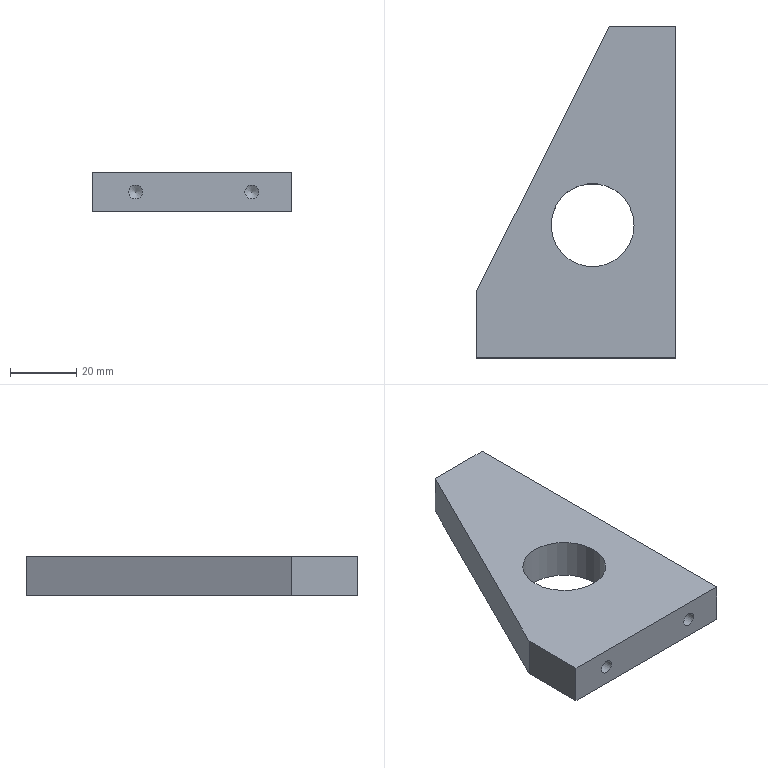Part | NX | 1 solid | 16 faces | box 60 x 100 x 12 mm | volume 45901 mm3 | plane 7 | cylinder 5 | cone 4 | commonest cylinder face diameters 4.2 x2 5 x2 25 x1
STEP:
#1=CARTESIAN_POINT('',(-30.,-30.,6.));
#2=VERTEX_POINT('',#1);
#3=CARTESIAN_POINT('',(-30.,-50.,6.));
#4=VERTEX_POINT('',#3);
#5=CARTESIAN_POINT('',(-30.,50.,6.));
#6=DIRECTION('',(0.,-1.,0.));
#7=VECTOR('',#6,1000.);
#8=LINE('',#5,#7);
#9=EDGE_CURVE('',#2,#4,#8,.T.);
#10=ORIENTED_EDGE('',*,*,#9,.F.);
#11=CARTESIAN_POINT('',(-30.,-30.,-6.));
#12=VERTEX_POINT('',#11);
#13=CARTESIAN_POINT('',(-30.,-30.,6.));
#14=DIRECTION('',(0.,0.,-1.));
#15=VECTOR('',#14,1000.);
#16=LINE('',#13,#15);
#17=EDGE_CURVE('',#2,#12,#16,.T.);
#18=ORIENTED_EDGE('',*,*,#17,.T.);
#19=CARTESIAN_POINT('',(-30.,-50.,-6.));
#20=VERTEX_POINT('',#19);
#21=CARTESIAN_POINT('',(-30.,50.,-6.));
#22=DIRECTION('',(0.,-1.,0.));
#23=VECTOR('',#22,1000.);
#24=LINE('',#21,#23);
#25=EDGE_CURVE('',#12,#20,#24,.T.);
#26=ORIENTED_EDGE('',*,*,#25,.T.);
#27=CARTESIAN_POINT('',(-30.,-50.,6.));
#28=DIRECTION('',(0.,0.,-1.));
#29=VECTOR('',#28,1000.);
#30=LINE('',#27,#29);
#31=EDGE_CURVE('',#4,#20,#30,.T.);
#32=ORIENTED_EDGE('',*,*,#31,.F.);
#33=EDGE_LOOP('',(#10,#18,#26,#32));
#34=FACE_BOUND('',#33,.T.);
#35=CARTESIAN_POINT('',(-30.,50.,6.));
#36=DIRECTION('',(1.,0.,0.));
#37=DIRECTION('',(0.,1.,0.));
#38=AXIS2_PLACEMENT_3D('',#35,#36,#37);
#39=PLANE('',#38);
#40=ADVANCED_FACE('',(#34),#39,.F.);
#41=CARTESIAN_POINT('',(18.,-50.,-2.1));
#42=VERTEX_POINT('',#41);
#43=CARTESIAN_POINT('',(18.,-50.,0.));
#44=DIRECTION('',(0.,-1.,0.));
#45=DIRECTION('',(0.,0.,-1.));
#46=AXIS2_PLACEMENT_3D('',#43,#44,#45);
#47=CIRCLE('',#46,2.1);
#48=EDGE_CURVE('',#42,#42,#47,.T.);
#49=ORIENTED_EDGE('',*,*,#48,.F.);
#50=EDGE_LOOP('',(#49));
#51=FACE_BOUND('',#50,.T.);
#52=CARTESIAN_POINT('',(-17.,-50.,-2.1));
#53=VERTEX_POINT('',#52);
#54=CARTESIAN_POINT('',(-17.,-50.,0.));
#55=DIRECTION('',(0.,-1.,0.));
#56=DIRECTION('',(0.,0.,-1.));
#57=AXIS2_PLACEMENT_3D('',#54,#55,#56);
#58=CIRCLE('',#57,2.1);
#59=EDGE_CURVE('',#53,#53,#58,.T.);
#60=ORIENTED_EDGE('',*,*,#59,.F.);
#61=EDGE_LOOP('',(#60));
#62=FACE_BOUND('',#61,.T.);
#63=CARTESIAN_POINT('',(30.,-50.,-6.));
#64=VERTEX_POINT('',#63);
#65=CARTESIAN_POINT('',(30.,-50.,-6.));
#66=DIRECTION('',(1.,0.,0.));
#67=VECTOR('',#66,1000.);
#68=LINE('',#65,#67);
#69=EDGE_CURVE('',#20,#64,#68,.T.);
#70=ORIENTED_EDGE('',*,*,#69,.T.);
#71=CARTESIAN_POINT('',(30.,-50.,6.));
#72=VERTEX_POINT('',#71);
#73=CARTESIAN_POINT('',(30.,-50.,6.));
#74=DIRECTION('',(0.,0.,-1.));
#75=VECTOR('',#74,1000.);
#76=LINE('',#73,#75);
#77=EDGE_CURVE('',#72,#64,#76,.T.);
#78=ORIENTED_EDGE('',*,*,#77,.F.);
#79=CARTESIAN_POINT('',(30.,-50.,6.));
#80=DIRECTION('',(1.,0.,0.));
#81=VECTOR('',#80,1000.);
#82=LINE('',#79,#81);
#83=EDGE_CURVE('',#4,#72,#82,.T.);
#84=ORIENTED_EDGE('',*,*,#83,.F.);
#85=ORIENTED_EDGE('',*,*,#31,.T.);
#86=EDGE_LOOP('',(#70,#78,#84,#85));
#87=FACE_BOUND('',#86,.T.);
#88=CARTESIAN_POINT('',(30.,-50.,6.));
#89=DIRECTION('',(0.,1.,0.));
#90=DIRECTION('',(-1.,0.,0.));
#91=AXIS2_PLACEMENT_3D('',#88,#89,#90);
#92=PLANE('',#91);
#93=ADVANCED_FACE('',(#51,#62,#87),#92,.F.);
#94=CARTESIAN_POINT('',(30.,35.,-2.5));
#95=VERTEX_POINT('',#94);
#96=CARTESIAN_POINT('',(30.,35.,0.));
#97=DIRECTION('',(1.,0.,0.));
#98=DIRECTION('',(0.,0.,-1.));
#99=AXIS2_PLACEMENT_3D('',#96,#97,#98);
#100=CIRCLE('',#99,2.5);
#101=EDGE_CURVE('',#95,#95,#100,.T.);
#102=ORIENTED_EDGE('',*,*,#101,.F.);
#103=EDGE_LOOP('',(#102));
#104=FACE_BOUND('',#103,.T.);
#105=CARTESIAN_POINT('',(30.,-30.,-2.5));
#106=VERTEX_POINT('',#105);
#107=CARTESIAN_POINT('',(30.,-30.,0.));
#108=DIRECTION('',(1.,0.,0.));
#109=DIRECTION('',(0.,0.,-1.));
#110=AXIS2_PLACEMENT_3D('',#107,#108,#109);
#111=CIRCLE('',#110,2.5);
#112=EDGE_CURVE('',#106,#106,#111,.T.);
#113=ORIENTED_EDGE('',*,*,#112,.F.);
#114=EDGE_LOOP('',(#113));
#115=FACE_BOUND('',#114,.T.);
#116=CARTESIAN_POINT('',(30.,50.,-6.));
#117=VERTEX_POINT('',#116);
#118=CARTESIAN_POINT('',(30.,50.,-6.));
#119=DIRECTION('',(0.,1.,0.));
#120=VECTOR('',#119,1000.);
#121=LINE('',#118,#120);
#122=EDGE_CURVE('',#64,#117,#121,.T.);
#123=ORIENTED_EDGE('',*,*,#122,.T.);
#124=CARTESIAN_POINT('',(30.,50.,6.));
#125=VERTEX_POINT('',#124);
#126=CARTESIAN_POINT('',(30.,50.,6.));
#127=DIRECTION('',(0.,0.,-1.));
#128=VECTOR('',#127,1000.);
#129=LINE('',#126,#128);
#130=EDGE_CURVE('',#125,#117,#129,.T.);
#131=ORIENTED_EDGE('',*,*,#130,.F.);
#132=CARTESIAN_POINT('',(30.,50.,6.));
#133=DIRECTION('',(0.,1.,0.));
#134=VECTOR('',#133,1000.);
#135=LINE('',#132,#134);
#136=EDGE_CURVE('',#72,#125,#135,.T.);
#137=ORIENTED_EDGE('',*,*,#136,.F.);
#138=ORIENTED_EDGE('',*,*,#77,.T.);
#139=EDGE_LOOP('',(#123,#131,#137,#138));
#140=FACE_BOUND('',#139,.T.);
#141=CARTESIAN_POINT('',(30.,50.,6.));
#142=DIRECTION('',(-1.,0.,0.));
#143=DIRECTION('',(0.,-1.,0.));
#144=AXIS2_PLACEMENT_3D('',#141,#142,#143);
#145=PLANE('',#144);
#146=ADVANCED_FACE('',(#104,#115,#140),#145,.F.);
#147=CARTESIAN_POINT('',(10.,50.,-6.));
#148=VERTEX_POINT('',#147);
#149=CARTESIAN_POINT('',(30.,50.,-6.));
#150=DIRECTION('',(-1.,0.,0.));
#151=VECTOR('',#150,1000.);
#152=LINE('',#149,#151);
#153=EDGE_CURVE('',#117,#148,#152,.T.);
#154=ORIENTED_EDGE('',*,*,#153,.T.);
#155=CARTESIAN_POINT('',(10.,50.,6.));
#156=VERTEX_POINT('',#155);
#157=CARTESIAN_POINT('',(10.,50.,6.));
#158=DIRECTION('',(0.,0.,1.));
#159=VECTOR('',#158,1000.);
#160=LINE('',#157,#159);
#161=EDGE_CURVE('',#148,#156,#160,.T.);
#162=ORIENTED_EDGE('',*,*,#161,.T.);
#163=CARTESIAN_POINT('',(30.,50.,6.));
#164=DIRECTION('',(-1.,0.,0.));
#165=VECTOR('',#164,1000.);
#166=LINE('',#163,#165);
#167=EDGE_CURVE('',#125,#156,#166,.T.);
#168=ORIENTED_EDGE('',*,*,#167,.F.);
#169=ORIENTED_EDGE('',*,*,#130,.T.);
#170=EDGE_LOOP('',(#154,#162,#168,#169));
#171=FACE_BOUND('',#170,.T.);
#172=CARTESIAN_POINT('',(30.,50.,6.));
#173=DIRECTION('',(0.,-1.,0.));
#174=DIRECTION('',(1.,0.,0.));
#175=AXIS2_PLACEMENT_3D('',#172,#173,#174);
#176=PLANE('',#175);
#177=ADVANCED_FACE('',(#171),#176,.F.);
#178=CARTESIAN_POINT('',(17.5,-10.,6.));
#179=VERTEX_POINT('',#178);
#180=CARTESIAN_POINT('',(5.,-10.,6.));
#181=DIRECTION('',(0.,0.,1.));
#182=DIRECTION('',(1.,0.,0.));
#183=AXIS2_PLACEMENT_3D('',#180,#181,#182);
#184=CIRCLE('',#183,12.5);
#185=EDGE_CURVE('',#179,#179,#184,.T.);
#186=ORIENTED_EDGE('',*,*,#185,.F.);
#187=EDGE_LOOP('',(#186));
#188=FACE_BOUND('',#187,.T.);
#189=ORIENTED_EDGE('',*,*,#167,.T.);
#190=CARTESIAN_POINT('',(-30.,-30.,6.));
#191=DIRECTION('',(0.4472,0.8944,0.));
#192=VECTOR('',#191,1000.);
#193=LINE('',#190,#192);
#194=EDGE_CURVE('',#156,#2,#193,.F.);
#195=ORIENTED_EDGE('',*,*,#194,.T.);
#196=ORIENTED_EDGE('',*,*,#9,.T.);
#197=ORIENTED_EDGE('',*,*,#83,.T.);
#198=ORIENTED_EDGE('',*,*,#136,.T.);
#199=EDGE_LOOP('',(#189,#195,#196,#197,#198));
#200=FACE_BOUND('',#199,.T.);
#201=CARTESIAN_POINT('',(0.,0.,6.));
#202=DIRECTION('',(0.,0.,-1.));
#203=DIRECTION('',(-1.,0.,0.));
#204=AXIS2_PLACEMENT_3D('',#201,#202,#203);
#205=PLANE('',#204);
#206=ADVANCED_FACE('',(#188,#200),#205,.F.);
#207=CARTESIAN_POINT('',(17.5,-10.,-6.));
#208=VERTEX_POINT('',#207);
#209=CARTESIAN_POINT('',(5.,-10.,-6.));
#210=DIRECTION('',(0.,0.,1.));
#211=DIRECTION('',(1.,0.,0.));
#212=AXIS2_PLACEMENT_3D('',#209,#210,#211);
#213=CIRCLE('',#212,12.5);
#214=EDGE_CURVE('',#208,#208,#213,.T.);
#215=ORIENTED_EDGE('',*,*,#214,.T.);
#216=EDGE_LOOP('',(#215));
#217=FACE_BOUND('',#216,.T.);
#218=ORIENTED_EDGE('',*,*,#25,.F.);
#219=CARTESIAN_POINT('',(-12.,6.,-6.));
#220=DIRECTION('',(-0.4472,-0.8944,0.));
#221=VECTOR('',#220,1000.);
#222=LINE('',#219,#221);
#223=EDGE_CURVE('',#12,#148,#222,.F.);
#224=ORIENTED_EDGE('',*,*,#223,.T.);
#225=ORIENTED_EDGE('',*,*,#153,.F.);
#226=ORIENTED_EDGE('',*,*,#122,.F.);
#227=ORIENTED_EDGE('',*,*,#69,.F.);
#228=EDGE_LOOP('',(#218,#224,#225,#226,#227));
#229=FACE_BOUND('',#228,.T.);
#230=CARTESIAN_POINT('',(0.,0.,-6.));
#231=DIRECTION('',(0.,0.,-1.));
#232=DIRECTION('',(-1.,0.,0.));
#233=AXIS2_PLACEMENT_3D('',#230,#231,#232);
#234=PLANE('',#233);
#235=ADVANCED_FACE('',(#217,#229),#234,.T.);
#236=CARTESIAN_POINT('',(13.498,-30.,0.));
#237=VERTEX_POINT('',#236);
#238=VERTEX_LOOP('',#237);
#239=FACE_BOUND('',#238,.T.);
#240=CARTESIAN_POINT('',(15.,-30.,-2.5));
#241=VERTEX_POINT('',#240);
#242=CARTESIAN_POINT('',(15.,-30.,0.));
#243=DIRECTION('',(1.,0.,0.));
#244=DIRECTION('',(0.,0.,-1.));
#245=AXIS2_PLACEMENT_3D('',#242,#243,#244);
#246=CIRCLE('',#245,2.5);
#247=EDGE_CURVE('',#241,#241,#246,.T.);
#248=ORIENTED_EDGE('',*,*,#247,.T.);
#249=EDGE_LOOP('',(#248));
#250=FACE_BOUND('',#249,.T.);
#251=CARTESIAN_POINT('',(15.,-30.,0.));
#252=DIRECTION('',(1.,0.,0.));
#253=DIRECTION('',(0.,0.,-1.));
#254=AXIS2_PLACEMENT_3D('',#251,#252,#253);
#255=CONICAL_SURFACE('',#254,2.5,1.03);
#256=ADVANCED_FACE('',(#239,#250),#255,.F.);
#257=ORIENTED_EDGE('',*,*,#247,.F.);
#258=EDGE_LOOP('',(#257));
#259=FACE_BOUND('',#258,.T.);
#260=ORIENTED_EDGE('',*,*,#112,.T.);
#261=EDGE_LOOP('',(#260));
#262=FACE_BOUND('',#261,.T.);
#263=CARTESIAN_POINT('',(30.,-30.,0.));
#264=DIRECTION('',(1.,0.,0.));
#265=DIRECTION('',(0.,0.,-1.));
#266=AXIS2_PLACEMENT_3D('',#263,#264,#265);
#267=CYLINDRICAL_SURFACE('',#266,2.5);
#268=ADVANCED_FACE('',(#259,#262),#267,.F.);
#269=CARTESIAN_POINT('',(13.498,35.,0.));
#270=VERTEX_POINT('',#269);
#271=VERTEX_LOOP('',#270);
#272=FACE_BOUND('',#271,.T.);
#273=CARTESIAN_POINT('',(15.,35.,-2.5));
#274=VERTEX_POINT('',#273);
#275=CARTESIAN_POINT('',(15.,35.,0.));
#276=DIRECTION('',(1.,0.,0.));
#277=DIRECTION('',(0.,0.,-1.));
#278=AXIS2_PLACEMENT_3D('',#275,#276,#277);
#279=CIRCLE('',#278,2.5);
#280=EDGE_CURVE('',#274,#274,#279,.T.);
#281=ORIENTED_EDGE('',*,*,#280,.T.);
#282=EDGE_LOOP('',(#281));
#283=FACE_BOUND('',#282,.T.);
#284=CARTESIAN_POINT('',(15.,35.,0.));
#285=DIRECTION('',(1.,0.,0.));
#286=DIRECTION('',(0.,0.,-1.));
#287=AXIS2_PLACEMENT_3D('',#284,#285,#286);
#288=CONICAL_SURFACE('',#287,2.5,1.03);
#289=ADVANCED_FACE('',(#272,#283),#288,.F.);
#290=ORIENTED_EDGE('',*,*,#280,.F.);
#291=EDGE_LOOP('',(#290));
#292=FACE_BOUND('',#291,.T.);
#293=ORIENTED_EDGE('',*,*,#101,.T.);
#294=EDGE_LOOP('',(#293));
#295=FACE_BOUND('',#294,.T.);
#296=CARTESIAN_POINT('',(30.,35.,0.));
#297=DIRECTION('',(1.,0.,0.));
#298=DIRECTION('',(0.,0.,-1.));
#299=AXIS2_PLACEMENT_3D('',#296,#297,#298);
#300=CYLINDRICAL_SURFACE('',#299,2.5);
#301=ADVANCED_FACE('',(#292,#295),#300,.F.);
#302=ORIENTED_EDGE('',*,*,#194,.F.);
#303=ORIENTED_EDGE('',*,*,#161,.F.);
#304=ORIENTED_EDGE('',*,*,#223,.F.);
#305=ORIENTED_EDGE('',*,*,#17,.F.);
#306=EDGE_LOOP('',(#302,#303,#304,#305));
#307=FACE_BOUND('',#306,.T.);
#308=CARTESIAN_POINT('',(-30.,-30.,6.));
#309=DIRECTION('',(0.8944,-0.4472,0.));
#310=DIRECTION('',(0.,0.,-1.));
#311=AXIS2_PLACEMENT_3D('',#308,#309,#310);
#312=PLANE('',#311);
#313=ADVANCED_FACE('',(#307),#312,.F.);
#314=CARTESIAN_POINT('',(-17.,-34.738,0.));
#315=VERTEX_POINT('',#314);
#316=VERTEX_LOOP('',#315);
#317=FACE_BOUND('',#316,.T.);
#318=CARTESIAN_POINT('',(-17.,-36.,-2.1));
#319=VERTEX_POINT('',#318);
#320=CARTESIAN_POINT('',(-17.,-36.,0.));
#321=DIRECTION('',(0.,-1.,0.));
#322=DIRECTION('',(0.,0.,-1.));
#323=AXIS2_PLACEMENT_3D('',#320,#321,#322);
#324=CIRCLE('',#323,2.1);
#325=EDGE_CURVE('',#319,#319,#324,.T.);
#326=ORIENTED_EDGE('',*,*,#325,.T.);
#327=EDGE_LOOP('',(#326));
#328=FACE_BOUND('',#327,.T.);
#329=CARTESIAN_POINT('',(-17.,-36.,0.));
#330=DIRECTION('',(0.,-1.,0.));
#331=DIRECTION('',(0.,0.,-1.));
#332=AXIS2_PLACEMENT_3D('',#329,#330,#331);
#333=CONICAL_SURFACE('',#332,2.1,1.03);
#334=ADVANCED_FACE('',(#317,#328),#333,.F.);
#335=ORIENTED_EDGE('',*,*,#325,.F.);
#336=EDGE_LOOP('',(#335));
#337=FACE_BOUND('',#336,.T.);
#338=ORIENTED_EDGE('',*,*,#59,.T.);
#339=EDGE_LOOP('',(#338));
#340=FACE_BOUND('',#339,.T.);
#341=CARTESIAN_POINT('',(-17.,-50.,0.));
#342=DIRECTION('',(0.,-1.,0.));
#343=DIRECTION('',(0.,0.,-1.));
#344=AXIS2_PLACEMENT_3D('',#341,#342,#343);
#345=CYLINDRICAL_SURFACE('',#344,2.1);
#346=ADVANCED_FACE('',(#337,#340),#345,.F.);
#347=CARTESIAN_POINT('',(18.,-34.738,0.));
#348=VERTEX_POINT('',#347);
#349=VERTEX_LOOP('',#348);
#350=FACE_BOUND('',#349,.T.);
#351=CARTESIAN_POINT('',(18.,-36.,-2.1));
#352=VERTEX_POINT('',#351);
#353=CARTESIAN_POINT('',(18.,-36.,0.));
#354=DIRECTION('',(0.,-1.,0.));
#355=DIRECTION('',(0.,0.,-1.));
#356=AXIS2_PLACEMENT_3D('',#353,#354,#355);
#357=CIRCLE('',#356,2.1);
#358=EDGE_CURVE('',#352,#352,#357,.T.);
#359=ORIENTED_EDGE('',*,*,#358,.T.);
#360=EDGE_LOOP('',(#359));
#361=FACE_BOUND('',#360,.T.);
#362=CARTESIAN_POINT('',(18.,-36.,0.));
#363=DIRECTION('',(0.,-1.,0.));
#364=DIRECTION('',(0.,0.,-1.));
#365=AXIS2_PLACEMENT_3D('',#362,#363,#364);
#366=CONICAL_SURFACE('',#365,2.1,1.03);
#367=ADVANCED_FACE('',(#350,#361),#366,.F.);
#368=ORIENTED_EDGE('',*,*,#358,.F.);
#369=EDGE_LOOP('',(#368));
#370=FACE_BOUND('',#369,.T.);
#371=ORIENTED_EDGE('',*,*,#48,.T.);
#372=EDGE_LOOP('',(#371));
#373=FACE_BOUND('',#372,.T.);
#374=CARTESIAN_POINT('',(18.,-50.,0.));
#375=DIRECTION('',(0.,-1.,0.));
#376=DIRECTION('',(0.,0.,-1.));
#377=AXIS2_PLACEMENT_3D('',#374,#375,#376);
#378=CYLINDRICAL_SURFACE('',#377,2.1);
#379=ADVANCED_FACE('',(#370,#373),#378,.F.);
#380=ORIENTED_EDGE('',*,*,#214,.F.);
#381=EDGE_LOOP('',(#380));
#382=FACE_BOUND('',#381,.T.);
#383=ORIENTED_EDGE('',*,*,#185,.T.);
#384=EDGE_LOOP('',(#383));
#385=FACE_BOUND('',#384,.T.);
#386=CARTESIAN_POINT('',(5.,-10.,-6.));
#387=DIRECTION('',(0.,0.,1.));
#388=DIRECTION('',(1.,0.,0.));
#389=AXIS2_PLACEMENT_3D('',#386,#387,#388);
#390=CYLINDRICAL_SURFACE('',#389,12.5);
#391=ADVANCED_FACE('',(#382,#385),#390,.F.);
#392=CLOSED_SHELL('',(#40,#93,#146,#177,#206,#235,#256,#268,#289,#301,#313,#334,#346,#367,#379,#391));
#393=MANIFOLD_SOLID_BREP('',#392);
#394=(LENGTH_UNIT()NAMED_UNIT(*)SI_UNIT(.MILLI.,.METRE.));
#395=UNCERTAINTY_MEASURE_WITH_UNIT(LENGTH_MEASURE(0.00001),#394,'','');
#396=(NAMED_UNIT(*)PLANE_ANGLE_UNIT()SI_UNIT($,.RADIAN.));
#397=(NAMED_UNIT(*)SI_UNIT($,.STERADIAN.)SOLID_ANGLE_UNIT());
#398=(GEOMETRIC_REPRESENTATION_CONTEXT(3)GLOBAL_UNCERTAINTY_ASSIGNED_CONTEXT((#395))GLOBAL_UNIT_ASSIGNED_CONTEXT((#394,#396,#397))REPRESENTATION_CONTEXT('',''));
#399=ADVANCED_BREP_SHAPE_REPRESENTATION('',(#393),#398);